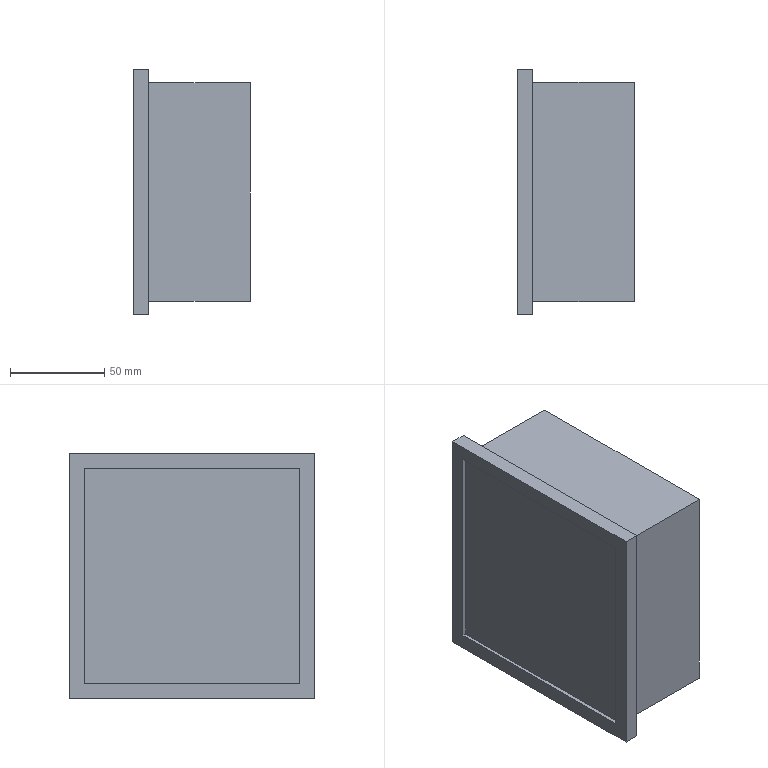Part | SolidWorks | features ICE 2, Extrusion 1 | 1 solid | 16 faces | box 62 x 130 x 130 mm | volume 835738 mm3 | plane 16
STEP:
#1=CARTESIAN_POINT('',(0.,-65.,-65.));
#2=VERTEX_POINT('',#1);
#3=CARTESIAN_POINT('',(0.,65.,-65.));
#4=VERTEX_POINT('',#3);
#5=CARTESIAN_POINT('',(0.,65.,-65.));
#6=DIRECTION('',(0.,1.,0.));
#7=VECTOR('',#6,1000.);
#8=LINE('',#5,#7);
#9=EDGE_CURVE('',#2,#4,#8,.T.);
#10=ORIENTED_EDGE('',*,*,#9,.T.);
#11=CARTESIAN_POINT('',(8.,65.,-65.));
#12=VERTEX_POINT('',#11);
#13=CARTESIAN_POINT('',(8.,65.,-65.));
#14=DIRECTION('',(-1.,0.,0.));
#15=VECTOR('',#14,1000.);
#16=LINE('',#13,#15);
#17=EDGE_CURVE('',#12,#4,#16,.T.);
#18=ORIENTED_EDGE('',*,*,#17,.F.);
#19=CARTESIAN_POINT('',(8.,-65.,-65.));
#20=VERTEX_POINT('',#19);
#21=CARTESIAN_POINT('',(8.,65.,-65.));
#22=DIRECTION('',(0.,1.,0.));
#23=VECTOR('',#22,1000.);
#24=LINE('',#21,#23);
#25=EDGE_CURVE('',#20,#12,#24,.T.);
#26=ORIENTED_EDGE('',*,*,#25,.F.);
#27=CARTESIAN_POINT('',(8.,-65.,-65.));
#28=DIRECTION('',(-1.,0.,0.));
#29=VECTOR('',#28,1000.);
#30=LINE('',#27,#29);
#31=EDGE_CURVE('',#20,#2,#30,.T.);
#32=ORIENTED_EDGE('',*,*,#31,.T.);
#33=EDGE_LOOP('',(#10,#18,#26,#32));
#34=FACE_OUTER_BOUND('',#33,.T.);
#35=CARTESIAN_POINT('',(8.,65.,-65.));
#36=DIRECTION('',(0.,0.,1.));
#37=DIRECTION('',(0.,-1.,0.));
#38=AXIS2_PLACEMENT_3D('',#35,#36,#37);
#39=PLANE('',#38);
#40=ADVANCED_FACE('',(#34),#39,.F.);
#41=CARTESIAN_POINT('',(0.,65.,65.));
#42=VERTEX_POINT('',#41);
#43=CARTESIAN_POINT('',(0.,65.,65.));
#44=DIRECTION('',(0.,0.,1.));
#45=VECTOR('',#44,1000.);
#46=LINE('',#43,#45);
#47=EDGE_CURVE('',#4,#42,#46,.T.);
#48=ORIENTED_EDGE('',*,*,#47,.T.);
#49=CARTESIAN_POINT('',(8.,65.,65.));
#50=VERTEX_POINT('',#49);
#51=CARTESIAN_POINT('',(8.,65.,65.));
#52=DIRECTION('',(-1.,0.,0.));
#53=VECTOR('',#52,1000.);
#54=LINE('',#51,#53);
#55=EDGE_CURVE('',#50,#42,#54,.T.);
#56=ORIENTED_EDGE('',*,*,#55,.F.);
#57=CARTESIAN_POINT('',(8.,65.,65.));
#58=DIRECTION('',(0.,0.,1.));
#59=VECTOR('',#58,1000.);
#60=LINE('',#57,#59);
#61=EDGE_CURVE('',#12,#50,#60,.T.);
#62=ORIENTED_EDGE('',*,*,#61,.F.);
#63=ORIENTED_EDGE('',*,*,#17,.T.);
#64=EDGE_LOOP('',(#48,#56,#62,#63));
#65=FACE_OUTER_BOUND('',#64,.T.);
#66=CARTESIAN_POINT('',(8.,65.,65.));
#67=DIRECTION('',(0.,-1.,0.));
#68=DIRECTION('',(0.,0.,-1.));
#69=AXIS2_PLACEMENT_3D('',#66,#67,#68);
#70=PLANE('',#69);
#71=ADVANCED_FACE('',(#65),#70,.F.);
#72=CARTESIAN_POINT('',(0.,-65.,65.));
#73=VERTEX_POINT('',#72);
#74=CARTESIAN_POINT('',(0.,65.,65.));
#75=DIRECTION('',(0.,-1.,0.));
#76=VECTOR('',#75,1000.);
#77=LINE('',#74,#76);
#78=EDGE_CURVE('',#42,#73,#77,.T.);
#79=ORIENTED_EDGE('',*,*,#78,.T.);
#80=CARTESIAN_POINT('',(8.,-65.,65.));
#81=VERTEX_POINT('',#80);
#82=CARTESIAN_POINT('',(8.,-65.,65.));
#83=DIRECTION('',(-1.,0.,0.));
#84=VECTOR('',#83,1000.);
#85=LINE('',#82,#84);
#86=EDGE_CURVE('',#81,#73,#85,.T.);
#87=ORIENTED_EDGE('',*,*,#86,.F.);
#88=CARTESIAN_POINT('',(8.,65.,65.));
#89=DIRECTION('',(0.,-1.,0.));
#90=VECTOR('',#89,1000.);
#91=LINE('',#88,#90);
#92=EDGE_CURVE('',#50,#81,#91,.T.);
#93=ORIENTED_EDGE('',*,*,#92,.F.);
#94=ORIENTED_EDGE('',*,*,#55,.T.);
#95=EDGE_LOOP('',(#79,#87,#93,#94));
#96=FACE_OUTER_BOUND('',#95,.T.);
#97=CARTESIAN_POINT('',(8.,65.,65.));
#98=DIRECTION('',(0.,0.,-1.));
#99=DIRECTION('',(0.,1.,0.));
#100=AXIS2_PLACEMENT_3D('',#97,#98,#99);
#101=PLANE('',#100);
#102=ADVANCED_FACE('',(#96),#101,.F.);
#103=CARTESIAN_POINT('',(0.,-65.,65.));
#104=DIRECTION('',(0.,0.,-1.));
#105=VECTOR('',#104,1000.);
#106=LINE('',#103,#105);
#107=EDGE_CURVE('',#73,#2,#106,.T.);
#108=ORIENTED_EDGE('',*,*,#107,.T.);
#109=ORIENTED_EDGE('',*,*,#31,.F.);
#110=CARTESIAN_POINT('',(8.,-65.,65.));
#111=DIRECTION('',(0.,0.,-1.));
#112=VECTOR('',#111,1000.);
#113=LINE('',#110,#112);
#114=EDGE_CURVE('',#81,#20,#113,.T.);
#115=ORIENTED_EDGE('',*,*,#114,.F.);
#116=ORIENTED_EDGE('',*,*,#86,.T.);
#117=EDGE_LOOP('',(#108,#109,#115,#116));
#118=FACE_OUTER_BOUND('',#117,.T.);
#119=CARTESIAN_POINT('',(8.,-65.,65.));
#120=DIRECTION('',(0.,1.,0.));
#121=DIRECTION('',(0.,0.,1.));
#122=AXIS2_PLACEMENT_3D('',#119,#120,#121);
#123=PLANE('',#122);
#124=ADVANCED_FACE('',(#118),#123,.F.);
#125=CARTESIAN_POINT('',(8.,-58.,-58.));
#126=VERTEX_POINT('',#125);
#127=CARTESIAN_POINT('',(8.,58.,-58.));
#128=VERTEX_POINT('',#127);
#129=CARTESIAN_POINT('',(8.,58.,-58.));
#130=DIRECTION('',(0.,1.,0.));
#131=VECTOR('',#130,1000.);
#132=LINE('',#129,#131);
#133=EDGE_CURVE('',#126,#128,#132,.T.);
#134=ORIENTED_EDGE('',*,*,#133,.F.);
#135=CARTESIAN_POINT('',(8.,-58.,58.));
#136=VERTEX_POINT('',#135);
#137=CARTESIAN_POINT('',(8.,-58.,58.));
#138=DIRECTION('',(0.,0.,-1.));
#139=VECTOR('',#138,1000.);
#140=LINE('',#137,#139);
#141=EDGE_CURVE('',#136,#126,#140,.T.);
#142=ORIENTED_EDGE('',*,*,#141,.F.);
#143=CARTESIAN_POINT('',(8.,58.,58.));
#144=VERTEX_POINT('',#143);
#145=CARTESIAN_POINT('',(8.,58.,58.));
#146=DIRECTION('',(0.,-1.,0.));
#147=VECTOR('',#146,1000.);
#148=LINE('',#145,#147);
#149=EDGE_CURVE('',#144,#136,#148,.T.);
#150=ORIENTED_EDGE('',*,*,#149,.F.);
#151=CARTESIAN_POINT('',(8.,58.,58.));
#152=DIRECTION('',(0.,0.,1.));
#153=VECTOR('',#152,1000.);
#154=LINE('',#151,#153);
#155=EDGE_CURVE('',#128,#144,#154,.T.);
#156=ORIENTED_EDGE('',*,*,#155,.F.);
#157=EDGE_LOOP('',(#134,#142,#150,#156));
#158=FACE_BOUND('',#157,.T.);
#159=ORIENTED_EDGE('',*,*,#25,.T.);
#160=ORIENTED_EDGE('',*,*,#61,.T.);
#161=ORIENTED_EDGE('',*,*,#92,.T.);
#162=ORIENTED_EDGE('',*,*,#114,.T.);
#163=EDGE_LOOP('',(#159,#160,#161,#162));
#164=FACE_OUTER_BOUND('',#163,.T.);
#165=CARTESIAN_POINT('',(8.,0.,0.));
#166=DIRECTION('',(1.,0.,0.));
#167=DIRECTION('',(0.,0.,-1.));
#168=AXIS2_PLACEMENT_3D('',#165,#166,#167);
#169=PLANE('',#168);
#170=ADVANCED_FACE('',(#158,#164),#169,.T.);
#171=CARTESIAN_POINT('',(0.,57.197,57.008));
#172=VERTEX_POINT('',#171);
#173=CARTESIAN_POINT('',(0.,57.197,-57.008));
#174=VERTEX_POINT('',#173);
#175=CARTESIAN_POINT('',(0.,57.197,-57.008));
#176=DIRECTION('',(0.,0.,-1.));
#177=VECTOR('',#176,1000.);
#178=LINE('',#175,#177);
#179=EDGE_CURVE('',#172,#174,#178,.T.);
#180=ORIENTED_EDGE('',*,*,#179,.F.);
#181=CARTESIAN_POINT('',(0.,-57.197,57.008));
#182=VERTEX_POINT('',#181);
#183=CARTESIAN_POINT('',(0.,57.197,57.008));
#184=DIRECTION('',(0.,1.,0.));
#185=VECTOR('',#184,1000.);
#186=LINE('',#183,#185);
#187=EDGE_CURVE('',#182,#172,#186,.T.);
#188=ORIENTED_EDGE('',*,*,#187,.F.);
#189=CARTESIAN_POINT('',(0.,-57.197,-57.008));
#190=VERTEX_POINT('',#189);
#191=CARTESIAN_POINT('',(0.,-57.197,-57.008));
#192=DIRECTION('',(0.,0.,1.));
#193=VECTOR('',#192,1000.);
#194=LINE('',#191,#193);
#195=EDGE_CURVE('',#190,#182,#194,.T.);
#196=ORIENTED_EDGE('',*,*,#195,.F.);
#197=CARTESIAN_POINT('',(0.,57.197,-57.008));
#198=DIRECTION('',(0.,-1.,0.));
#199=VECTOR('',#198,1000.);
#200=LINE('',#197,#199);
#201=EDGE_CURVE('',#174,#190,#200,.T.);
#202=ORIENTED_EDGE('',*,*,#201,.F.);
#203=EDGE_LOOP('',(#180,#188,#196,#202));
#204=FACE_BOUND('',#203,.T.);
#205=ORIENTED_EDGE('',*,*,#9,.F.);
#206=ORIENTED_EDGE('',*,*,#107,.F.);
#207=ORIENTED_EDGE('',*,*,#78,.F.);
#208=ORIENTED_EDGE('',*,*,#47,.F.);
#209=EDGE_LOOP('',(#205,#206,#207,#208));
#210=FACE_OUTER_BOUND('',#209,.T.);
#211=CARTESIAN_POINT('',(0.,0.,0.));
#212=DIRECTION('',(1.,0.,0.));
#213=DIRECTION('',(0.,0.,-1.));
#214=AXIS2_PLACEMENT_3D('',#211,#212,#213);
#215=PLANE('',#214);
#216=ADVANCED_FACE('',(#204,#210),#215,.F.);
#217=ORIENTED_EDGE('',*,*,#133,.T.);
#218=CARTESIAN_POINT('',(62.,58.,-58.));
#219=VERTEX_POINT('',#218);
#220=CARTESIAN_POINT('',(62.,58.,-58.));
#221=DIRECTION('',(-1.,0.,0.));
#222=VECTOR('',#221,1000.);
#223=LINE('',#220,#222);
#224=EDGE_CURVE('',#219,#128,#223,.T.);
#225=ORIENTED_EDGE('',*,*,#224,.F.);
#226=CARTESIAN_POINT('',(62.,-58.,-58.));
#227=VERTEX_POINT('',#226);
#228=CARTESIAN_POINT('',(62.,58.,-58.));
#229=DIRECTION('',(0.,1.,0.));
#230=VECTOR('',#229,1000.);
#231=LINE('',#228,#230);
#232=EDGE_CURVE('',#227,#219,#231,.T.);
#233=ORIENTED_EDGE('',*,*,#232,.F.);
#234=CARTESIAN_POINT('',(62.,-58.,-58.));
#235=DIRECTION('',(-1.,0.,0.));
#236=VECTOR('',#235,1000.);
#237=LINE('',#234,#236);
#238=EDGE_CURVE('',#227,#126,#237,.T.);
#239=ORIENTED_EDGE('',*,*,#238,.T.);
#240=EDGE_LOOP('',(#217,#225,#233,#239));
#241=FACE_OUTER_BOUND('',#240,.T.);
#242=CARTESIAN_POINT('',(62.,58.,-58.));
#243=DIRECTION('',(0.,0.,1.));
#244=DIRECTION('',(0.,-1.,0.));
#245=AXIS2_PLACEMENT_3D('',#242,#243,#244);
#246=PLANE('',#245);
#247=ADVANCED_FACE('',(#241),#246,.F.);
#248=ORIENTED_EDGE('',*,*,#155,.T.);
#249=CARTESIAN_POINT('',(62.,58.,58.));
#250=VERTEX_POINT('',#249);
#251=CARTESIAN_POINT('',(62.,58.,58.));
#252=DIRECTION('',(-1.,0.,0.));
#253=VECTOR('',#252,1000.);
#254=LINE('',#251,#253);
#255=EDGE_CURVE('',#250,#144,#254,.T.);
#256=ORIENTED_EDGE('',*,*,#255,.F.);
#257=CARTESIAN_POINT('',(62.,58.,58.));
#258=DIRECTION('',(0.,0.,1.));
#259=VECTOR('',#258,1000.);
#260=LINE('',#257,#259);
#261=EDGE_CURVE('',#219,#250,#260,.T.);
#262=ORIENTED_EDGE('',*,*,#261,.F.);
#263=ORIENTED_EDGE('',*,*,#224,.T.);
#264=EDGE_LOOP('',(#248,#256,#262,#263));
#265=FACE_OUTER_BOUND('',#264,.T.);
#266=CARTESIAN_POINT('',(62.,58.,58.));
#267=DIRECTION('',(0.,-1.,0.));
#268=DIRECTION('',(0.,0.,-1.));
#269=AXIS2_PLACEMENT_3D('',#266,#267,#268);
#270=PLANE('',#269);
#271=ADVANCED_FACE('',(#265),#270,.F.);
#272=ORIENTED_EDGE('',*,*,#149,.T.);
#273=CARTESIAN_POINT('',(62.,-58.,58.));
#274=VERTEX_POINT('',#273);
#275=CARTESIAN_POINT('',(62.,-58.,58.));
#276=DIRECTION('',(-1.,0.,0.));
#277=VECTOR('',#276,1000.);
#278=LINE('',#275,#277);
#279=EDGE_CURVE('',#274,#136,#278,.T.);
#280=ORIENTED_EDGE('',*,*,#279,.F.);
#281=CARTESIAN_POINT('',(62.,58.,58.));
#282=DIRECTION('',(0.,-1.,0.));
#283=VECTOR('',#282,1000.);
#284=LINE('',#281,#283);
#285=EDGE_CURVE('',#250,#274,#284,.T.);
#286=ORIENTED_EDGE('',*,*,#285,.F.);
#287=ORIENTED_EDGE('',*,*,#255,.T.);
#288=EDGE_LOOP('',(#272,#280,#286,#287));
#289=FACE_OUTER_BOUND('',#288,.T.);
#290=CARTESIAN_POINT('',(62.,58.,58.));
#291=DIRECTION('',(0.,0.,-1.));
#292=DIRECTION('',(0.,1.,0.));
#293=AXIS2_PLACEMENT_3D('',#290,#291,#292);
#294=PLANE('',#293);
#295=ADVANCED_FACE('',(#289),#294,.F.);
#296=ORIENTED_EDGE('',*,*,#141,.T.);
#297=ORIENTED_EDGE('',*,*,#238,.F.);
#298=CARTESIAN_POINT('',(62.,-58.,58.));
#299=DIRECTION('',(0.,0.,-1.));
#300=VECTOR('',#299,1000.);
#301=LINE('',#298,#300);
#302=EDGE_CURVE('',#274,#227,#301,.T.);
#303=ORIENTED_EDGE('',*,*,#302,.F.);
#304=ORIENTED_EDGE('',*,*,#279,.T.);
#305=EDGE_LOOP('',(#296,#297,#303,#304));
#306=FACE_OUTER_BOUND('',#305,.T.);
#307=CARTESIAN_POINT('',(62.,-58.,58.));
#308=DIRECTION('',(0.,1.,0.));
#309=DIRECTION('',(0.,0.,1.));
#310=AXIS2_PLACEMENT_3D('',#307,#308,#309);
#311=PLANE('',#310);
#312=ADVANCED_FACE('',(#306),#311,.F.);
#313=ORIENTED_EDGE('',*,*,#232,.T.);
#314=ORIENTED_EDGE('',*,*,#261,.T.);
#315=ORIENTED_EDGE('',*,*,#285,.T.);
#316=ORIENTED_EDGE('',*,*,#302,.T.);
#317=EDGE_LOOP('',(#313,#314,#315,#316));
#318=FACE_OUTER_BOUND('',#317,.T.);
#319=CARTESIAN_POINT('',(62.,0.,0.));
#320=DIRECTION('',(1.,0.,0.));
#321=DIRECTION('',(0.,0.,-1.));
#322=AXIS2_PLACEMENT_3D('',#319,#320,#321);
#323=PLANE('',#322);
#324=ADVANCED_FACE('',(#318),#323,.T.);
#325=ORIENTED_EDGE('',*,*,#187,.T.);
#326=CARTESIAN_POINT('',(2.,57.197,57.008));
#327=VERTEX_POINT('',#326);
#328=CARTESIAN_POINT('',(2.,57.197,57.008));
#329=DIRECTION('',(-1.,0.,0.));
#330=VECTOR('',#329,1000.);
#331=LINE('',#328,#330);
#332=EDGE_CURVE('',#327,#172,#331,.T.);
#333=ORIENTED_EDGE('',*,*,#332,.F.);
#334=CARTESIAN_POINT('',(2.,-57.197,57.008));
#335=VERTEX_POINT('',#334);
#336=CARTESIAN_POINT('',(2.,57.197,57.008));
#337=DIRECTION('',(0.,1.,0.));
#338=VECTOR('',#337,1000.);
#339=LINE('',#336,#338);
#340=EDGE_CURVE('',#335,#327,#339,.T.);
#341=ORIENTED_EDGE('',*,*,#340,.F.);
#342=CARTESIAN_POINT('',(2.,-57.197,57.008));
#343=DIRECTION('',(-1.,0.,0.));
#344=VECTOR('',#343,1000.);
#345=LINE('',#342,#344);
#346=EDGE_CURVE('',#335,#182,#345,.T.);
#347=ORIENTED_EDGE('',*,*,#346,.T.);
#348=EDGE_LOOP('',(#325,#333,#341,#347));
#349=FACE_OUTER_BOUND('',#348,.T.);
#350=CARTESIAN_POINT('',(2.,57.197,57.008));
#351=DIRECTION('',(0.,0.,1.));
#352=DIRECTION('',(1.,0.,0.));
#353=AXIS2_PLACEMENT_3D('',#350,#351,#352);
#354=PLANE('',#353);
#355=ADVANCED_FACE('',(#349),#354,.F.);
#356=ORIENTED_EDGE('',*,*,#195,.T.);
#357=ORIENTED_EDGE('',*,*,#346,.F.);
#358=CARTESIAN_POINT('',(2.,-57.197,-57.008));
#359=VERTEX_POINT('',#358);
#360=CARTESIAN_POINT('',(2.,-57.197,-57.008));
#361=DIRECTION('',(0.,0.,1.));
#362=VECTOR('',#361,1000.);
#363=LINE('',#360,#362);
#364=EDGE_CURVE('',#359,#335,#363,.T.);
#365=ORIENTED_EDGE('',*,*,#364,.F.);
#366=CARTESIAN_POINT('',(2.,-57.197,-57.008));
#367=DIRECTION('',(-1.,0.,0.));
#368=VECTOR('',#367,1000.);
#369=LINE('',#366,#368);
#370=EDGE_CURVE('',#359,#190,#369,.T.);
#371=ORIENTED_EDGE('',*,*,#370,.T.);
#372=EDGE_LOOP('',(#356,#357,#365,#371));
#373=FACE_OUTER_BOUND('',#372,.T.);
#374=CARTESIAN_POINT('',(2.,-57.197,-57.008));
#375=DIRECTION('',(0.,-1.,0.));
#376=DIRECTION('',(0.,0.,-1.));
#377=AXIS2_PLACEMENT_3D('',#374,#375,#376);
#378=PLANE('',#377);
#379=ADVANCED_FACE('',(#373),#378,.F.);
#380=ORIENTED_EDGE('',*,*,#201,.T.);
#381=ORIENTED_EDGE('',*,*,#370,.F.);
#382=CARTESIAN_POINT('',(2.,57.197,-57.008));
#383=VERTEX_POINT('',#382);
#384=CARTESIAN_POINT('',(2.,57.197,-57.008));
#385=DIRECTION('',(0.,-1.,0.));
#386=VECTOR('',#385,1000.);
#387=LINE('',#384,#386);
#388=EDGE_CURVE('',#383,#359,#387,.T.);
#389=ORIENTED_EDGE('',*,*,#388,.F.);
#390=CARTESIAN_POINT('',(2.,57.197,-57.008));
#391=DIRECTION('',(-1.,0.,0.));
#392=VECTOR('',#391,1000.);
#393=LINE('',#390,#392);
#394=EDGE_CURVE('',#383,#174,#393,.T.);
#395=ORIENTED_EDGE('',*,*,#394,.T.);
#396=EDGE_LOOP('',(#380,#381,#389,#395));
#397=FACE_OUTER_BOUND('',#396,.T.);
#398=CARTESIAN_POINT('',(2.,57.197,-57.008));
#399=DIRECTION('',(0.,0.,-1.));
#400=DIRECTION('',(-1.,0.,0.));
#401=AXIS2_PLACEMENT_3D('',#398,#399,#400);
#402=PLANE('',#401);
#403=ADVANCED_FACE('',(#397),#402,.F.);
#404=ORIENTED_EDGE('',*,*,#179,.T.);
#405=ORIENTED_EDGE('',*,*,#394,.F.);
#406=CARTESIAN_POINT('',(2.,57.197,-57.008));
#407=DIRECTION('',(0.,0.,-1.));
#408=VECTOR('',#407,1000.);
#409=LINE('',#406,#408);
#410=EDGE_CURVE('',#327,#383,#409,.T.);
#411=ORIENTED_EDGE('',*,*,#410,.F.);
#412=ORIENTED_EDGE('',*,*,#332,.T.);
#413=EDGE_LOOP('',(#404,#405,#411,#412));
#414=FACE_OUTER_BOUND('',#413,.T.);
#415=CARTESIAN_POINT('',(2.,57.197,-57.008));
#416=DIRECTION('',(0.,1.,0.));
#417=DIRECTION('',(0.,0.,1.));
#418=AXIS2_PLACEMENT_3D('',#415,#416,#417);
#419=PLANE('',#418);
#420=ADVANCED_FACE('',(#414),#419,.F.);
#421=ORIENTED_EDGE('',*,*,#340,.T.);
#422=ORIENTED_EDGE('',*,*,#410,.T.);
#423=ORIENTED_EDGE('',*,*,#388,.T.);
#424=ORIENTED_EDGE('',*,*,#364,.T.);
#425=EDGE_LOOP('',(#421,#422,#423,#424));
#426=FACE_OUTER_BOUND('',#425,.T.);
#427=CARTESIAN_POINT('',(2.,0.,0.));
#428=DIRECTION('',(-1.,0.,0.));
#429=DIRECTION('',(0.,0.,1.));
#430=AXIS2_PLACEMENT_3D('',#427,#428,#429);
#431=PLANE('',#430);
#432=ADVANCED_FACE('',(#426),#431,.T.);
#433=CLOSED_SHELL('',(#40,#71,#102,#124,#170,#216,#247,#271,#295,#312,#324,#355,#379,#403,#420,#432));
#434=MANIFOLD_SOLID_BREP('',#433);
#435=CARTESIAN_POINT('',(0.,0.,0.));
#436=DIRECTION('',(0.,0.,1.));
#437=DIRECTION('',(1.,0.,0.));
#438=AXIS2_PLACEMENT_3D('',#435,#436,#437);
#439=(LENGTH_UNIT()NAMED_UNIT(*)SI_UNIT(.MILLI.,.METRE.));
#440=UNCERTAINTY_MEASURE_WITH_UNIT(LENGTH_MEASURE(0.00001),#439,'','');
#441=(NAMED_UNIT(*)PLANE_ANGLE_UNIT()SI_UNIT($,.RADIAN.));
#442=(NAMED_UNIT(*)SI_UNIT($,.STERADIAN.)SOLID_ANGLE_UNIT());
#443=(GEOMETRIC_REPRESENTATION_CONTEXT(3)GLOBAL_UNCERTAINTY_ASSIGNED_CONTEXT((#440))GLOBAL_UNIT_ASSIGNED_CONTEXT((#439,#441,#442))REPRESENTATION_CONTEXT('',''));
#444=ADVANCED_BREP_SHAPE_REPRESENTATION('',(#434,#438),#443);